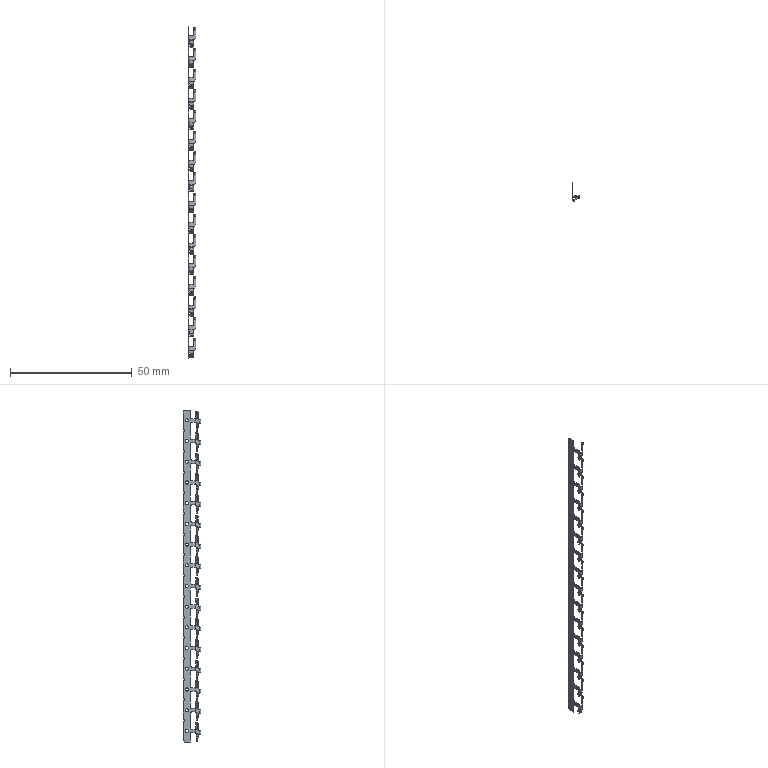Part | NX | 1 solid | 1670 faces | box 2.994 x 7.25 x 136.3 mm | volume 181.604 mm3 | plane 726 | cylinder 624 | torus 256 | sphere 64 | commonest cylinder face diameters 0.2 x112 0.4 x112 0.5 x96 0.7 x64 0.6 x48 1 x48